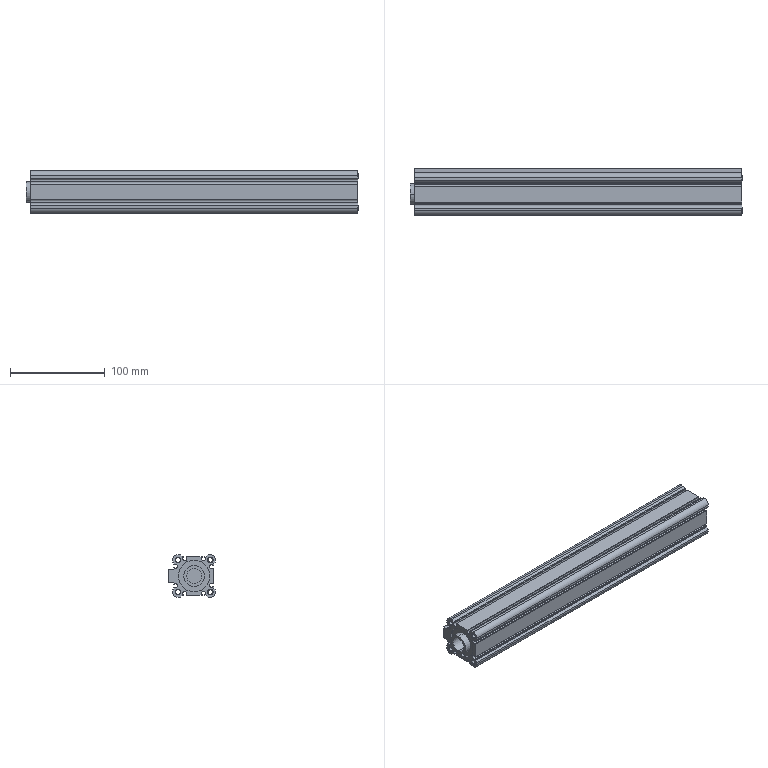Part | SolidWorks | features BaseBody 1 | 1 solid | 145 faces | box 350.5 x 49.5 x 45 mm | volume 322350 mm3 | plane 65 | cylinder 60 | cone 20 | commonest cylinder face diameters 4.26 x18 4.917 x16 6 x8 8.566 x4 11 x4 33.4 x4